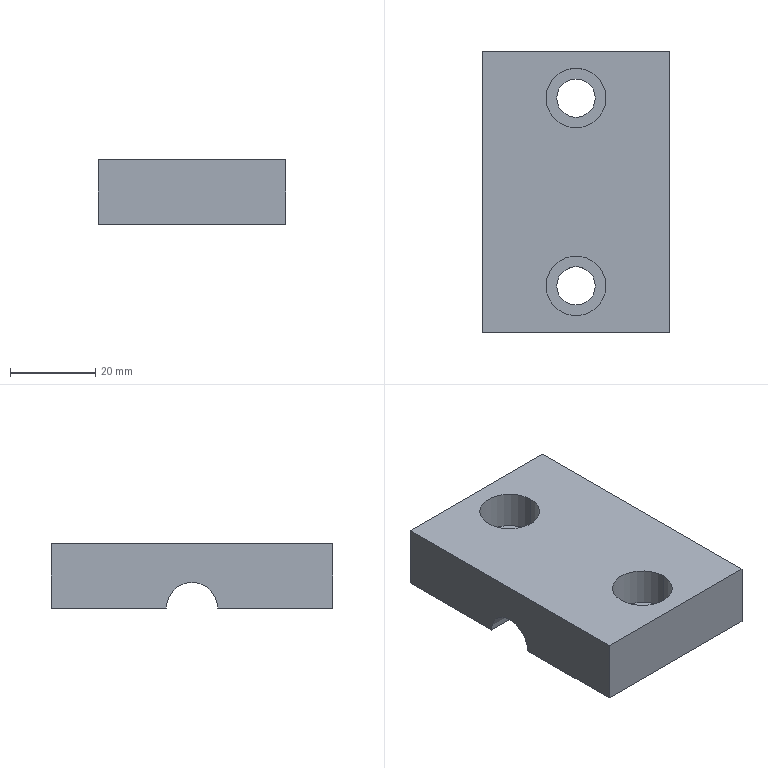Part | 1 solid | 18 faces | box 44 x 66 x 15 mm | volume 37538 mm3 | plane 9 | cylinder 9 | commonest cylinder face diameters 9 x4 14 x4 12 x1
STEP:
#1=CARTESIAN_POINT('',(0.,0.,0.));
#2=DIRECTION('',(0.,0.,1.));
#3=DIRECTION('',(1.,0.,0.));
#4=AXIS2_PLACEMENT_3D('',#1,#2,#3);
#5=CARTESIAN_POINT('',(-499.933,163.5,-310.6));
#6=VERTEX_POINT('',#5);
#7=CARTESIAN_POINT('',(-508.933,163.5,-310.6));
#8=VERTEX_POINT('',#7);
#9=CARTESIAN_POINT('',(-504.433,163.5,-310.6));
#10=DIRECTION('',(0.,0.,-1.));
#11=DIRECTION('',(-1.,0.,0.));
#12=AXIS2_PLACEMENT_3D('',#9,#10,#11);
#13=CIRCLE('',#12,4.5);
#14=CARTESIAN_POINT('',(-504.433,141.5,-310.6));
#15=DIRECTION('',(0.,0.,1.));
#16=DIRECTION('',(-1.,0.,0.));
#17=AXIS2_PLACEMENT_3D('',#14,#15,#16);
#18=PLANE('',#17);
#19=CARTESIAN_POINT('',(4.5,-22.));
#20=CARTESIAN_POINT('',(4.5,-29.794));
#21=CARTESIAN_POINT('',(-2.25,-25.897));
#22=CARTESIAN_POINT('',(-9.,-22.));
#23=CARTESIAN_POINT('',(-2.25,-18.103));
#24=CARTESIAN_POINT('',(4.5,-14.206));
#25=CARTESIAN_POINT('',(4.5,-22.));
#26=(BOUNDED_CURVE()B_SPLINE_CURVE(2,(#19,#20,#21,#22,#23,#24,#25),.UNSPECIFIED.,.T.,.F.)B_SPLINE_CURVE_WITH_KNOTS((1,2,2,2,2,1),(-2.094,0.,2.094,4.189,6.283,8.378),.UNSPECIFIED.)CURVE()GEOMETRIC_REPRESENTATION_ITEM()RATIONAL_B_SPLINE_CURVE((1.,0.5,1.,0.5,1.,0.5,1.))REPRESENTATION_ITEM(''));
#27=(GEOMETRIC_REPRESENTATION_CONTEXT(2)PARAMETRIC_REPRESENTATION_CONTEXT()REPRESENTATION_CONTEXT('',''));
#28=DEFINITIONAL_REPRESENTATION('',(#26),#27);
#29=PCURVE('',#18,#28);
#30=CARTESIAN_POINT('',(-504.433,163.5,-422.6));
#31=DIRECTION('',(0.,0.,1.));
#32=DIRECTION('',(0.,1.,0.));
#33=AXIS2_PLACEMENT_3D('',#30,#31,#32);
#34=CYLINDRICAL_SURFACE('',#33,4.5);
#35=CARTESIAN_POINT('',(7.854,112.));
#36=DIRECTION('',(-1.,0.));
#37=VECTOR('',#36,1.);
#38=LINE('',#35,#37);
#39=(GEOMETRIC_REPRESENTATION_CONTEXT(2)PARAMETRIC_REPRESENTATION_CONTEXT()REPRESENTATION_CONTEXT('',''));
#40=DEFINITIONAL_REPRESENTATION('',(#38),#39);
#41=PCURVE('',#34,#40);
#42=SURFACE_CURVE('',#13,(#29,#41),.PCURVE_S1.);
#43=EDGE_CURVE('',#6,#8,#42,.T.);
#44=ORIENTED_EDGE('',*,*,#43,.F.);
#45=CARTESIAN_POINT('',(-504.433,163.5,-310.6));
#46=DIRECTION('',(0.,0.,-1.));
#47=DIRECTION('',(-1.,0.,0.));
#48=AXIS2_PLACEMENT_3D('',#45,#46,#47);
#49=CIRCLE('',#48,4.5);
#50=CARTESIAN_POINT('',(4.5,-22.));
#51=CARTESIAN_POINT('',(4.5,-29.794));
#52=CARTESIAN_POINT('',(-2.25,-25.897));
#53=CARTESIAN_POINT('',(-9.,-22.));
#54=CARTESIAN_POINT('',(-2.25,-18.103));
#55=CARTESIAN_POINT('',(4.5,-14.206));
#56=CARTESIAN_POINT('',(4.5,-22.));
#57=(BOUNDED_CURVE()B_SPLINE_CURVE(2,(#50,#51,#52,#53,#54,#55,#56),.UNSPECIFIED.,.T.,.F.)B_SPLINE_CURVE_WITH_KNOTS((1,2,2,2,2,1),(-2.094,0.,2.094,4.189,6.283,8.378),.UNSPECIFIED.)CURVE()GEOMETRIC_REPRESENTATION_ITEM()RATIONAL_B_SPLINE_CURVE((1.,0.5,1.,0.5,1.,0.5,1.))REPRESENTATION_ITEM(''));
#58=(GEOMETRIC_REPRESENTATION_CONTEXT(2)PARAMETRIC_REPRESENTATION_CONTEXT()REPRESENTATION_CONTEXT('',''));
#59=DEFINITIONAL_REPRESENTATION('',(#57),#58);
#60=PCURVE('',#18,#59);
#61=CARTESIAN_POINT('',(-504.433,163.5,-422.6));
#62=DIRECTION('',(0.,0.,1.));
#63=DIRECTION('',(0.,-1.,0.));
#64=AXIS2_PLACEMENT_3D('',#61,#62,#63);
#65=CYLINDRICAL_SURFACE('',#64,4.5);
#66=CARTESIAN_POINT('',(4.712,112.));
#67=DIRECTION('',(-1.,0.));
#68=VECTOR('',#67,1.);
#69=LINE('',#66,#68);
#70=(GEOMETRIC_REPRESENTATION_CONTEXT(2)PARAMETRIC_REPRESENTATION_CONTEXT()REPRESENTATION_CONTEXT('',''));
#71=DEFINITIONAL_REPRESENTATION('',(#69),#70);
#72=PCURVE('',#65,#71);
#73=SURFACE_CURVE('',#49,(#60,#72),.PCURVE_S1.);
#74=EDGE_CURVE('',#8,#6,#73,.T.);
#75=ORIENTED_EDGE('',*,*,#74,.F.);
#76=EDGE_LOOP('',(#44,#75));
#77=FACE_BOUND('',#76,.T.);
#78=CARTESIAN_POINT('',(-482.433,147.5,-310.6));
#79=VERTEX_POINT('',#78);
#80=CARTESIAN_POINT('',(-482.433,174.5,-310.6));
#81=VERTEX_POINT('',#80);
#82=CARTESIAN_POINT('',(-482.433,141.5,-310.6));
#83=DIRECTION('',(0.,1.,0.));
#84=VECTOR('',#83,1.);
#85=LINE('',#82,#84);
#86=CARTESIAN_POINT('',(-22.,0.));
#87=DIRECTION('',(0.,-1.));
#88=VECTOR('',#87,1.);
#89=LINE('',#86,#88);
#90=(GEOMETRIC_REPRESENTATION_CONTEXT(2)PARAMETRIC_REPRESENTATION_CONTEXT()REPRESENTATION_CONTEXT('',''));
#91=DEFINITIONAL_REPRESENTATION('',(#89),#90);
#92=PCURVE('',#18,#91);
#93=CARTESIAN_POINT('',(-482.433,141.5,-319.1));
#94=DIRECTION('',(1.,0.,0.));
#95=DIRECTION('',(0.,0.,1.));
#96=AXIS2_PLACEMENT_3D('',#93,#94,#95);
#97=PLANE('',#96);
#98=CARTESIAN_POINT('',(8.5,0.));
#99=DIRECTION('',(0.,-1.));
#100=VECTOR('',#99,1.);
#101=LINE('',#98,#100);
#102=(GEOMETRIC_REPRESENTATION_CONTEXT(2)PARAMETRIC_REPRESENTATION_CONTEXT()REPRESENTATION_CONTEXT('',''));
#103=DEFINITIONAL_REPRESENTATION('',(#101),#102);
#104=PCURVE('',#97,#103);
#105=SURFACE_CURVE('',#85,(#92,#104),.PCURVE_S1.);
#106=EDGE_CURVE('',#79,#81,#105,.T.);
#107=ORIENTED_EDGE('',*,*,#106,.F.);
#108=CARTESIAN_POINT('',(-526.433,147.5,-310.6));
#109=VERTEX_POINT('',#108);
#110=CARTESIAN_POINT('',(-517.416,147.5,-310.6));
#111=DIRECTION('',(-1.,0.,0.));
#112=VECTOR('',#111,1.);
#113=LINE('',#110,#112);
#114=CARTESIAN_POINT('',(12.983,-6.));
#115=DIRECTION('',(1.,0.));
#116=VECTOR('',#115,1.);
#117=LINE('',#114,#116);
#118=(GEOMETRIC_REPRESENTATION_CONTEXT(2)PARAMETRIC_REPRESENTATION_CONTEXT()REPRESENTATION_CONTEXT('',''));
#119=DEFINITIONAL_REPRESENTATION('',(#117),#118);
#120=PCURVE('',#18,#119);
#121=CARTESIAN_POINT('',(-517.416,141.5,-310.6));
#122=DIRECTION('',(-1.,0.,0.));
#123=DIRECTION('',(0.,0.,-1.));
#124=AXIS2_PLACEMENT_3D('',#121,#122,#123);
#125=CYLINDRICAL_SURFACE('',#124,6.);
#126=CARTESIAN_POINT('',(4.712,0.));
#127=DIRECTION('',(0.,1.));
#128=VECTOR('',#127,1.);
#129=LINE('',#126,#128);
#130=(GEOMETRIC_REPRESENTATION_CONTEXT(2)PARAMETRIC_REPRESENTATION_CONTEXT()REPRESENTATION_CONTEXT('',''));
#131=DEFINITIONAL_REPRESENTATION('',(#129),#130);
#132=PCURVE('',#125,#131);
#133=SURFACE_CURVE('',#113,(#120,#132),.PCURVE_S1.);
#134=EDGE_CURVE('',#79,#109,#133,.T.);
#135=ORIENTED_EDGE('',*,*,#134,.T.);
#136=CARTESIAN_POINT('',(-526.433,174.5,-310.6));
#137=VERTEX_POINT('',#136);
#138=CARTESIAN_POINT('',(-526.433,141.5,-310.6));
#139=DIRECTION('',(0.,-1.,0.));
#140=VECTOR('',#139,1.);
#141=LINE('',#138,#140);
#142=CARTESIAN_POINT('',(22.,0.));
#143=DIRECTION('',(0.,1.));
#144=VECTOR('',#143,1.);
#145=LINE('',#142,#144);
#146=(GEOMETRIC_REPRESENTATION_CONTEXT(2)PARAMETRIC_REPRESENTATION_CONTEXT()REPRESENTATION_CONTEXT('',''));
#147=DEFINITIONAL_REPRESENTATION('',(#145),#146);
#148=PCURVE('',#18,#147);
#149=CARTESIAN_POINT('',(-526.433,141.5,-319.1));
#150=DIRECTION('',(-1.,0.,0.));
#151=DIRECTION('',(0.,0.,-1.));
#152=AXIS2_PLACEMENT_3D('',#149,#150,#151);
#153=PLANE('',#152);
#154=CARTESIAN_POINT('',(-8.5,0.));
#155=DIRECTION('',(0.,1.));
#156=VECTOR('',#155,1.);
#157=LINE('',#154,#156);
#158=(GEOMETRIC_REPRESENTATION_CONTEXT(2)PARAMETRIC_REPRESENTATION_CONTEXT()REPRESENTATION_CONTEXT('',''));
#159=DEFINITIONAL_REPRESENTATION('',(#157),#158);
#160=PCURVE('',#153,#159);
#161=SURFACE_CURVE('',#141,(#148,#160),.PCURVE_S1.);
#162=EDGE_CURVE('',#137,#109,#161,.T.);
#163=ORIENTED_EDGE('',*,*,#162,.F.);
#164=CARTESIAN_POINT('',(-504.433,174.5,-310.6));
#165=DIRECTION('',(1.,0.,0.));
#166=VECTOR('',#165,1.);
#167=LINE('',#164,#166);
#168=CARTESIAN_POINT('',(0.,-33.));
#169=DIRECTION('',(-1.,0.));
#170=VECTOR('',#169,1.);
#171=LINE('',#168,#170);
#172=(GEOMETRIC_REPRESENTATION_CONTEXT(2)PARAMETRIC_REPRESENTATION_CONTEXT()REPRESENTATION_CONTEXT('',''));
#173=DEFINITIONAL_REPRESENTATION('',(#171),#172);
#174=PCURVE('',#18,#173);
#175=CARTESIAN_POINT('',(-504.433,174.5,-319.1));
#176=DIRECTION('',(0.,1.,0.));
#177=DIRECTION('',(0.,0.,-1.));
#178=AXIS2_PLACEMENT_3D('',#175,#176,#177);
#179=PLANE('',#178);
#180=CARTESIAN_POINT('',(-8.5,0.));
#181=DIRECTION('',(0.,-1.));
#182=VECTOR('',#181,1.);
#183=LINE('',#180,#182);
#184=(GEOMETRIC_REPRESENTATION_CONTEXT(2)PARAMETRIC_REPRESENTATION_CONTEXT()REPRESENTATION_CONTEXT('',''));
#185=DEFINITIONAL_REPRESENTATION('',(#183),#184);
#186=PCURVE('',#179,#185);
#187=SURFACE_CURVE('',#167,(#174,#186),.PCURVE_S1.);
#188=EDGE_CURVE('',#137,#81,#187,.T.);
#189=ORIENTED_EDGE('',*,*,#188,.T.);
#190=EDGE_LOOP('',(#107,#135,#163,#189));
#191=FACE_BOUND('',#190,.T.);
#192=ADVANCED_FACE('',(#77,#191),#18,.F.);
#193=ORIENTED_EDGE('',*,*,#188,.F.);
#194=CARTESIAN_POINT('',(-526.433,174.5,-295.6));
#195=VERTEX_POINT('',#194);
#196=CARTESIAN_POINT('',(-526.433,174.5,-319.1));
#197=DIRECTION('',(0.,0.,1.));
#198=VECTOR('',#197,1.);
#199=LINE('',#196,#198);
#200=CARTESIAN_POINT('',(0.,22.));
#201=DIRECTION('',(-1.,0.));
#202=VECTOR('',#201,1.);
#203=LINE('',#200,#202);
#204=(GEOMETRIC_REPRESENTATION_CONTEXT(2)PARAMETRIC_REPRESENTATION_CONTEXT()REPRESENTATION_CONTEXT('',''));
#205=DEFINITIONAL_REPRESENTATION('',(#203),#204);
#206=PCURVE('',#179,#205);
#207=CARTESIAN_POINT('',(0.,-33.));
#208=DIRECTION('',(-1.,0.));
#209=VECTOR('',#208,1.);
#210=LINE('',#207,#209);
#211=(GEOMETRIC_REPRESENTATION_CONTEXT(2)PARAMETRIC_REPRESENTATION_CONTEXT()REPRESENTATION_CONTEXT('',''));
#212=DEFINITIONAL_REPRESENTATION('',(#210),#211);
#213=PCURVE('',#153,#212);
#214=SURFACE_CURVE('',#199,(#206,#213),.PCURVE_S1.);
#215=EDGE_CURVE('',#137,#195,#214,.T.);
#216=ORIENTED_EDGE('',*,*,#215,.T.);
#217=CARTESIAN_POINT('',(-482.433,174.5,-295.6));
#218=VERTEX_POINT('',#217);
#219=CARTESIAN_POINT('',(-504.433,174.5,-295.6));
#220=DIRECTION('',(1.,0.,0.));
#221=VECTOR('',#220,1.);
#222=LINE('',#219,#221);
#223=CARTESIAN_POINT('',(-23.5,0.));
#224=DIRECTION('',(0.,-1.));
#225=VECTOR('',#224,1.);
#226=LINE('',#223,#225);
#227=(GEOMETRIC_REPRESENTATION_CONTEXT(2)PARAMETRIC_REPRESENTATION_CONTEXT()REPRESENTATION_CONTEXT('',''));
#228=DEFINITIONAL_REPRESENTATION('',(#226),#227);
#229=PCURVE('',#179,#228);
#230=CARTESIAN_POINT('',(-504.433,141.5,-295.6));
#231=DIRECTION('',(0.,0.,1.));
#232=DIRECTION('',(-1.,0.,0.));
#233=AXIS2_PLACEMENT_3D('',#230,#231,#232);
#234=PLANE('',#233);
#235=CARTESIAN_POINT('',(0.,-33.));
#236=DIRECTION('',(-1.,0.));
#237=VECTOR('',#236,1.);
#238=LINE('',#235,#237);
#239=(GEOMETRIC_REPRESENTATION_CONTEXT(2)PARAMETRIC_REPRESENTATION_CONTEXT()REPRESENTATION_CONTEXT('',''));
#240=DEFINITIONAL_REPRESENTATION('',(#238),#239);
#241=PCURVE('',#234,#240);
#242=SURFACE_CURVE('',#222,(#229,#241),.PCURVE_S1.);
#243=EDGE_CURVE('',#195,#218,#242,.T.);
#244=ORIENTED_EDGE('',*,*,#243,.T.);
#245=CARTESIAN_POINT('',(-482.433,174.5,-319.1));
#246=DIRECTION('',(0.,0.,1.));
#247=VECTOR('',#246,1.);
#248=LINE('',#245,#247);
#249=CARTESIAN_POINT('',(0.,-22.));
#250=DIRECTION('',(-1.,0.));
#251=VECTOR('',#250,1.);
#252=LINE('',#249,#251);
#253=(GEOMETRIC_REPRESENTATION_CONTEXT(2)PARAMETRIC_REPRESENTATION_CONTEXT()REPRESENTATION_CONTEXT('',''));
#254=DEFINITIONAL_REPRESENTATION('',(#252),#253);
#255=PCURVE('',#179,#254);
#256=CARTESIAN_POINT('',(0.,-33.));
#257=DIRECTION('',(1.,0.));
#258=VECTOR('',#257,1.);
#259=LINE('',#256,#258);
#260=(GEOMETRIC_REPRESENTATION_CONTEXT(2)PARAMETRIC_REPRESENTATION_CONTEXT()REPRESENTATION_CONTEXT('',''));
#261=DEFINITIONAL_REPRESENTATION('',(#259),#260);
#262=PCURVE('',#97,#261);
#263=SURFACE_CURVE('',#248,(#255,#262),.PCURVE_S1.);
#264=EDGE_CURVE('',#81,#218,#263,.T.);
#265=ORIENTED_EDGE('',*,*,#264,.F.);
#266=EDGE_LOOP('',(#193,#216,#244,#265));
#267=FACE_BOUND('',#266,.T.);
#268=ADVANCED_FACE('',(#267),#179,.T.);
#269=CARTESIAN_POINT('',(-482.433,108.5,-310.6));
#270=VERTEX_POINT('',#269);
#271=CARTESIAN_POINT('',(-482.433,135.5,-310.6));
#272=VERTEX_POINT('',#271);
#273=CARTESIAN_POINT('',(-482.433,141.5,-310.6));
#274=DIRECTION('',(0.,1.,0.));
#275=VECTOR('',#274,1.);
#276=LINE('',#273,#275);
#277=CARTESIAN_POINT('',(8.5,0.));
#278=DIRECTION('',(0.,-1.));
#279=VECTOR('',#278,1.);
#280=LINE('',#277,#279);
#281=(GEOMETRIC_REPRESENTATION_CONTEXT(2)PARAMETRIC_REPRESENTATION_CONTEXT()REPRESENTATION_CONTEXT('',''));
#282=DEFINITIONAL_REPRESENTATION('',(#280),#281);
#283=PCURVE('',#97,#282);
#284=CARTESIAN_POINT('',(-504.433,141.5,-310.6));
#285=DIRECTION('',(0.,0.,1.));
#286=DIRECTION('',(-1.,0.,0.));
#287=AXIS2_PLACEMENT_3D('',#284,#285,#286);
#288=PLANE('',#287);
#289=CARTESIAN_POINT('',(-22.,0.));
#290=DIRECTION('',(0.,-1.));
#291=VECTOR('',#290,1.);
#292=LINE('',#289,#291);
#293=(GEOMETRIC_REPRESENTATION_CONTEXT(2)PARAMETRIC_REPRESENTATION_CONTEXT()REPRESENTATION_CONTEXT('',''));
#294=DEFINITIONAL_REPRESENTATION('',(#292),#293);
#295=PCURVE('',#288,#294);
#296=SURFACE_CURVE('',#276,(#283,#295),.PCURVE_S1.);
#297=EDGE_CURVE('',#270,#272,#296,.T.);
#298=ORIENTED_EDGE('',*,*,#297,.T.);
#299=CARTESIAN_POINT('',(-482.433,141.5,-310.6));
#300=DIRECTION('',(1.,0.,0.));
#301=DIRECTION('',(0.,0.,-1.));
#302=AXIS2_PLACEMENT_3D('',#299,#300,#301);
#303=CIRCLE('',#302,6.);
#304=CARTESIAN_POINT('',(8.5,0.));
#305=DIRECTION('',(-1.,0.));
#306=AXIS2_PLACEMENT_2D('',#304,#305);
#307=CIRCLE('',#306,6.);
#308=(GEOMETRIC_REPRESENTATION_CONTEXT(2)PARAMETRIC_REPRESENTATION_CONTEXT()REPRESENTATION_CONTEXT('',''));
#309=DEFINITIONAL_REPRESENTATION('',(#307),#308);
#310=PCURVE('',#97,#309);
#311=CARTESIAN_POINT('',(6.283,-34.983));
#312=DIRECTION('',(-1.,0.));
#313=VECTOR('',#312,1.);
#314=LINE('',#311,#313);
#315=(GEOMETRIC_REPRESENTATION_CONTEXT(2)PARAMETRIC_REPRESENTATION_CONTEXT()REPRESENTATION_CONTEXT('',''));
#316=DEFINITIONAL_REPRESENTATION('',(#314),#315);
#317=PCURVE('',#125,#316);
#318=SURFACE_CURVE('',#303,(#310,#317),.PCURVE_S1.);
#319=EDGE_CURVE('',#79,#272,#318,.T.);
#320=ORIENTED_EDGE('',*,*,#319,.F.);
#321=ORIENTED_EDGE('',*,*,#106,.T.);
#322=ORIENTED_EDGE('',*,*,#264,.T.);
#323=CARTESIAN_POINT('',(-482.433,108.5,-295.6));
#324=VERTEX_POINT('',#323);
#325=CARTESIAN_POINT('',(-482.433,141.5,-295.6));
#326=DIRECTION('',(0.,1.,0.));
#327=VECTOR('',#326,1.);
#328=LINE('',#325,#327);
#329=CARTESIAN_POINT('',(23.5,0.));
#330=DIRECTION('',(0.,-1.));
#331=VECTOR('',#330,1.);
#332=LINE('',#329,#331);
#333=(GEOMETRIC_REPRESENTATION_CONTEXT(2)PARAMETRIC_REPRESENTATION_CONTEXT()REPRESENTATION_CONTEXT('',''));
#334=DEFINITIONAL_REPRESENTATION('',(#332),#333);
#335=PCURVE('',#97,#334);
#336=CARTESIAN_POINT('',(-22.,0.));
#337=DIRECTION('',(0.,-1.));
#338=VECTOR('',#337,1.);
#339=LINE('',#336,#338);
#340=(GEOMETRIC_REPRESENTATION_CONTEXT(2)PARAMETRIC_REPRESENTATION_CONTEXT()REPRESENTATION_CONTEXT('',''));
#341=DEFINITIONAL_REPRESENTATION('',(#339),#340);
#342=PCURVE('',#234,#341);
#343=SURFACE_CURVE('',#328,(#335,#342),.PCURVE_S1.);
#344=EDGE_CURVE('',#324,#218,#343,.T.);
#345=ORIENTED_EDGE('',*,*,#344,.F.);
#346=CARTESIAN_POINT('',(-482.433,108.5,-319.1));
#347=DIRECTION('',(0.,0.,1.));
#348=VECTOR('',#347,1.);
#349=LINE('',#346,#348);
#350=CARTESIAN_POINT('',(0.,33.));
#351=DIRECTION('',(1.,0.));
#352=VECTOR('',#351,1.);
#353=LINE('',#350,#352);
#354=(GEOMETRIC_REPRESENTATION_CONTEXT(2)PARAMETRIC_REPRESENTATION_CONTEXT()REPRESENTATION_CONTEXT('',''));
#355=DEFINITIONAL_REPRESENTATION('',(#353),#354);
#356=PCURVE('',#97,#355);
#357=CARTESIAN_POINT('',(-504.433,108.5,-319.1));
#358=DIRECTION('',(0.,-1.,0.));
#359=DIRECTION('',(0.,0.,-1.));
#360=AXIS2_PLACEMENT_3D('',#357,#358,#359);
#361=PLANE('',#360);
#362=CARTESIAN_POINT('',(0.,22.));
#363=DIRECTION('',(-1.,0.));
#364=VECTOR('',#363,1.);
#365=LINE('',#362,#364);
#366=(GEOMETRIC_REPRESENTATION_CONTEXT(2)PARAMETRIC_REPRESENTATION_CONTEXT()REPRESENTATION_CONTEXT('',''));
#367=DEFINITIONAL_REPRESENTATION('',(#365),#366);
#368=PCURVE('',#361,#367);
#369=SURFACE_CURVE('',#349,(#356,#368),.PCURVE_S1.);
#370=EDGE_CURVE('',#270,#324,#369,.T.);
#371=ORIENTED_EDGE('',*,*,#370,.F.);
#372=EDGE_LOOP('',(#298,#320,#321,#322,#345,#371));
#373=FACE_BOUND('',#372,.T.);
#374=ADVANCED_FACE('',(#373),#97,.T.);
#375=CARTESIAN_POINT('',(-526.433,108.5,-310.6));
#376=VERTEX_POINT('',#375);
#377=CARTESIAN_POINT('',(-504.433,108.5,-310.6));
#378=DIRECTION('',(1.,0.,0.));
#379=VECTOR('',#378,1.);
#380=LINE('',#377,#379);
#381=CARTESIAN_POINT('',(-8.5,0.));
#382=DIRECTION('',(0.,1.));
#383=VECTOR('',#382,1.);
#384=LINE('',#381,#383);
#385=(GEOMETRIC_REPRESENTATION_CONTEXT(2)PARAMETRIC_REPRESENTATION_CONTEXT()REPRESENTATION_CONTEXT('',''));
#386=DEFINITIONAL_REPRESENTATION('',(#384),#385);
#387=PCURVE('',#361,#386);
#388=CARTESIAN_POINT('',(0.,33.));
#389=DIRECTION('',(-1.,0.));
#390=VECTOR('',#389,1.);
#391=LINE('',#388,#390);
#392=(GEOMETRIC_REPRESENTATION_CONTEXT(2)PARAMETRIC_REPRESENTATION_CONTEXT()REPRESENTATION_CONTEXT('',''));
#393=DEFINITIONAL_REPRESENTATION('',(#391),#392);
#394=PCURVE('',#288,#393);
#395=SURFACE_CURVE('',#380,(#387,#394),.PCURVE_S1.);
#396=EDGE_CURVE('',#376,#270,#395,.T.);
#397=ORIENTED_EDGE('',*,*,#396,.T.);
#398=ORIENTED_EDGE('',*,*,#370,.T.);
#399=CARTESIAN_POINT('',(-526.433,108.5,-295.6));
#400=VERTEX_POINT('',#399);
#401=CARTESIAN_POINT('',(-504.433,108.5,-295.6));
#402=DIRECTION('',(1.,0.,0.));
#403=VECTOR('',#402,1.);
#404=LINE('',#401,#403);
#405=CARTESIAN_POINT('',(-23.5,0.));
#406=DIRECTION('',(0.,1.));
#407=VECTOR('',#406,1.);
#408=LINE('',#405,#407);
#409=(GEOMETRIC_REPRESENTATION_CONTEXT(2)PARAMETRIC_REPRESENTATION_CONTEXT()REPRESENTATION_CONTEXT('',''));
#410=DEFINITIONAL_REPRESENTATION('',(#408),#409);
#411=PCURVE('',#361,#410);
#412=CARTESIAN_POINT('',(0.,33.));
#413=DIRECTION('',(-1.,0.));
#414=VECTOR('',#413,1.);
#415=LINE('',#412,#414);
#416=(GEOMETRIC_REPRESENTATION_CONTEXT(2)PARAMETRIC_REPRESENTATION_CONTEXT()REPRESENTATION_CONTEXT('',''));
#417=DEFINITIONAL_REPRESENTATION('',(#415),#416);
#418=PCURVE('',#234,#417);
#419=SURFACE_CURVE('',#404,(#411,#418),.PCURVE_S1.);
#420=EDGE_CURVE('',#400,#324,#419,.T.);
#421=ORIENTED_EDGE('',*,*,#420,.F.);
#422=CARTESIAN_POINT('',(-526.433,108.5,-319.1));
#423=DIRECTION('',(0.,0.,1.));
#424=VECTOR('',#423,1.);
#425=LINE('',#422,#424);
#426=CARTESIAN_POINT('',(0.,-22.));
#427=DIRECTION('',(-1.,0.));
#428=VECTOR('',#427,1.);
#429=LINE('',#426,#428);
#430=(GEOMETRIC_REPRESENTATION_CONTEXT(2)PARAMETRIC_REPRESENTATION_CONTEXT()REPRESENTATION_CONTEXT('',''));
#431=DEFINITIONAL_REPRESENTATION('',(#429),#430);
#432=PCURVE('',#361,#431);
#433=CARTESIAN_POINT('',(0.,33.));
#434=DIRECTION('',(-1.,0.));
#435=VECTOR('',#434,1.);
#436=LINE('',#433,#435);
#437=(GEOMETRIC_REPRESENTATION_CONTEXT(2)PARAMETRIC_REPRESENTATION_CONTEXT()REPRESENTATION_CONTEXT('',''));
#438=DEFINITIONAL_REPRESENTATION('',(#436),#437);
#439=PCURVE('',#153,#438);
#440=SURFACE_CURVE('',#425,(#432,#439),.PCURVE_S1.);
#441=EDGE_CURVE('',#376,#400,#440,.T.);
#442=ORIENTED_EDGE('',*,*,#441,.F.);
#443=EDGE_LOOP('',(#397,#398,#421,#442));
#444=FACE_BOUND('',#443,.T.);
#445=ADVANCED_FACE('',(#444),#361,.T.);
#446=CARTESIAN_POINT('',(-526.433,135.5,-310.6));
#447=VERTEX_POINT('',#446);
#448=CARTESIAN_POINT('',(-526.433,141.5,-310.6));
#449=DIRECTION('',(0.,-1.,0.));
#450=VECTOR('',#449,1.);
#451=LINE('',#448,#450);
#452=CARTESIAN_POINT('',(-8.5,0.));
#453=DIRECTION('',(0.,1.));
#454=VECTOR('',#453,1.);
#455=LINE('',#452,#454);
#456=(GEOMETRIC_REPRESENTATION_CONTEXT(2)PARAMETRIC_REPRESENTATION_CONTEXT()REPRESENTATION_CONTEXT('',''));
#457=DEFINITIONAL_REPRESENTATION('',(#455),#456);
#458=PCURVE('',#153,#457);
#459=CARTESIAN_POINT('',(22.,0.));
#460=DIRECTION('',(0.,1.));
#461=VECTOR('',#460,1.);
#462=LINE('',#459,#461);
#463=(GEOMETRIC_REPRESENTATION_CONTEXT(2)PARAMETRIC_REPRESENTATION_CONTEXT()REPRESENTATION_CONTEXT('',''));
#464=DEFINITIONAL_REPRESENTATION('',(#462),#463);
#465=PCURVE('',#288,#464);
#466=SURFACE_CURVE('',#451,(#458,#465),.PCURVE_S1.);
#467=EDGE_CURVE('',#447,#376,#466,.T.);
#468=ORIENTED_EDGE('',*,*,#467,.T.);
#469=ORIENTED_EDGE('',*,*,#441,.T.);
#470=CARTESIAN_POINT('',(-526.433,141.5,-295.6));
#471=DIRECTION('',(0.,-1.,0.));
#472=VECTOR('',#471,1.);
#473=LINE('',#470,#472);
#474=CARTESIAN_POINT('',(-23.5,0.));
#475=DIRECTION('',(0.,1.));
#476=VECTOR('',#475,1.);
#477=LINE('',#474,#476);
#478=(GEOMETRIC_REPRESENTATION_CONTEXT(2)PARAMETRIC_REPRESENTATION_CONTEXT()REPRESENTATION_CONTEXT('',''));
#479=DEFINITIONAL_REPRESENTATION('',(#477),#478);
#480=PCURVE('',#153,#479);
#481=CARTESIAN_POINT('',(22.,0.));
#482=DIRECTION('',(0.,1.));
#483=VECTOR('',#482,1.);
#484=LINE('',#481,#483);
#485=(GEOMETRIC_REPRESENTATION_CONTEXT(2)PARAMETRIC_REPRESENTATION_CONTEXT()REPRESENTATION_CONTEXT('',''));
#486=DEFINITIONAL_REPRESENTATION('',(#484),#485);
#487=PCURVE('',#234,#486);
#488=SURFACE_CURVE('',#473,(#480,#487),.PCURVE_S1.);
#489=EDGE_CURVE('',#195,#400,#488,.T.);
#490=ORIENTED_EDGE('',*,*,#489,.F.);
#491=ORIENTED_EDGE('',*,*,#215,.F.);
#492=ORIENTED_EDGE('',*,*,#162,.T.);
#493=CARTESIAN_POINT('',(-526.433,141.5,-310.6));
#494=DIRECTION('',(-1.,0.,0.));
#495=DIRECTION('',(0.,0.,1.));
#496=AXIS2_PLACEMENT_3D('',#493,#494,#495);
#497=CIRCLE('',#496,6.);
#498=CARTESIAN_POINT('',(-8.5,0.));
#499=DIRECTION('',(-1.,0.));
#500=AXIS2_PLACEMENT_2D('',#498,#499);
#501=CIRCLE('',#500,6.);
#502=(GEOMETRIC_REPRESENTATION_CONTEXT(2)PARAMETRIC_REPRESENTATION_CONTEXT()REPRESENTATION_CONTEXT('',''));
#503=DEFINITIONAL_REPRESENTATION('',(#501),#502);
#504=PCURVE('',#153,#503);
#505=CARTESIAN_POINT('',(-3.142,9.017));
#506=DIRECTION('',(1.,0.));
#507=VECTOR('',#506,1.);
#508=LINE('',#505,#507);
#509=(GEOMETRIC_REPRESENTATION_CONTEXT(2)PARAMETRIC_REPRESENTATION_CONTEXT()REPRESENTATION_CONTEXT('',''));
#510=DEFINITIONAL_REPRESENTATION('',(#508),#509);
#511=PCURVE('',#125,#510);
#512=SURFACE_CURVE('',#497,(#504,#511),.PCURVE_S1.);
#513=EDGE_CURVE('',#447,#109,#512,.T.);
#514=ORIENTED_EDGE('',*,*,#513,.F.);
#515=EDGE_LOOP('',(#468,#469,#490,#491,#492,#514));
#516=FACE_BOUND('',#515,.T.);
#517=ADVANCED_FACE('',(#516),#153,.T.);
#518=ORIENTED_EDGE('',*,*,#134,.T.);
#519=ORIENTED_EDGE('',*,*,#513,.F.);
#520=CARTESIAN_POINT('',(-517.416,135.5,-310.6));
#521=DIRECTION('',(1.,0.,0.));
#522=VECTOR('',#521,1.);
#523=LINE('',#520,#522);
#524=CARTESIAN_POINT('',(1.571,0.));
#525=DIRECTION('',(0.,-1.));
#526=VECTOR('',#525,1.);
#527=LINE('',#524,#526);
#528=(GEOMETRIC_REPRESENTATION_CONTEXT(2)PARAMETRIC_REPRESENTATION_CONTEXT()REPRESENTATION_CONTEXT('',''));
#529=DEFINITIONAL_REPRESENTATION('',(#527),#528);
#530=PCURVE('',#125,#529);
#531=CARTESIAN_POINT('',(12.983,6.));
#532=DIRECTION('',(-1.,0.));
#533=VECTOR('',#532,1.);
#534=LINE('',#531,#533);
#535=(GEOMETRIC_REPRESENTATION_CONTEXT(2)PARAMETRIC_REPRESENTATION_CONTEXT()REPRESENTATION_CONTEXT('',''));
#536=DEFINITIONAL_REPRESENTATION('',(#534),#535);
#537=PCURVE('',#288,#536);
#538=SURFACE_CURVE('',#523,(#530,#537),.PCURVE_S1.);
#539=EDGE_CURVE('',#447,#272,#538,.T.);
#540=ORIENTED_EDGE('',*,*,#539,.T.);
#541=ORIENTED_EDGE('',*,*,#319,.F.);
#542=EDGE_LOOP('',(#518,#519,#540,#541));
#543=FACE_BOUND('',#542,.F.);
#544=ADVANCED_FACE('',(#543),#125,.F.);
#545=CARTESIAN_POINT('',(-508.933,119.5,-310.6));
#546=VERTEX_POINT('',#545);
#547=CARTESIAN_POINT('',(-499.933,119.5,-310.6));
#548=VERTEX_POINT('',#547);
#549=CARTESIAN_POINT('',(-504.433,119.5,-310.6));
#550=DIRECTION('',(0.,0.,1.));
#551=DIRECTION('',(-1.,0.,0.));
#552=AXIS2_PLACEMENT_3D('',#549,#550,#551);
#553=CIRCLE('',#552,4.5);
#554=CARTESIAN_POINT('',(0.,22.));
#555=DIRECTION('',(1.,0.));
#556=AXIS2_PLACEMENT_2D('',#554,#555);
#557=CIRCLE('',#556,4.5);
#558=(GEOMETRIC_REPRESENTATION_CONTEXT(2)PARAMETRIC_REPRESENTATION_CONTEXT()REPRESENTATION_CONTEXT('',''));
#559=DEFINITIONAL_REPRESENTATION('',(#557),#558);
#560=PCURVE('',#288,#559);
#561=CARTESIAN_POINT('',(-504.433,119.5,-422.6));
#562=DIRECTION('',(0.,0.,1.));
#563=DIRECTION('',(0.,1.,0.));
#564=AXIS2_PLACEMENT_3D('',#561,#562,#563);
#565=CYLINDRICAL_SURFACE('',#564,4.5);
#566=CARTESIAN_POINT('',(1.571,112.));
#567=DIRECTION('',(1.,0.));
#568=VECTOR('',#567,1.);
#569=LINE('',#566,#568);
#570=(GEOMETRIC_REPRESENTATION_CONTEXT(2)PARAMETRIC_REPRESENTATION_CONTEXT()REPRESENTATION_CONTEXT('',''));
#571=DEFINITIONAL_REPRESENTATION('',(#569),#570);
#572=PCURVE('',#565,#571);
#573=SURFACE_CURVE('',#553,(#560,#572),.PCURVE_S1.);
#574=EDGE_CURVE('',#546,#548,#573,.T.);
#575=ORIENTED_EDGE('',*,*,#574,.T.);
#576=CARTESIAN_POINT('',(-504.433,119.5,-310.6));
#577=DIRECTION('',(0.,0.,1.));
#578=DIRECTION('',(-1.,0.,0.));
#579=AXIS2_PLACEMENT_3D('',#576,#577,#578);
#580=CIRCLE('',#579,4.5);
#581=CARTESIAN_POINT('',(0.,22.));
#582=DIRECTION('',(1.,0.));
#583=AXIS2_PLACEMENT_2D('',#581,#582);
#584=CIRCLE('',#583,4.5);
#585=(GEOMETRIC_REPRESENTATION_CONTEXT(2)PARAMETRIC_REPRESENTATION_CONTEXT()REPRESENTATION_CONTEXT('',''));
#586=DEFINITIONAL_REPRESENTATION('',(#584),#585);
#587=PCURVE('',#288,#586);
#588=CARTESIAN_POINT('',(-504.433,119.5,-422.6));
#589=DIRECTION('',(0.,0.,1.));
#590=DIRECTION('',(0.,-1.,0.));
#591=AXIS2_PLACEMENT_3D('',#588,#589,#590);
#592=CYLINDRICAL_SURFACE('',#591,4.5);
#593=CARTESIAN_POINT('',(-1.571,112.));
#594=DIRECTION('',(1.,0.));
#595=VECTOR('',#594,1.);
#596=LINE('',#593,#595);
#597=(GEOMETRIC_REPRESENTATION_CONTEXT(2)PARAMETRIC_REPRESENTATION_CONTEXT()REPRESENTATION_CONTEXT('',''));
#598=DEFINITIONAL_REPRESENTATION('',(#596),#597);
#599=PCURVE('',#592,#598);
#600=SURFACE_CURVE('',#580,(#587,#599),.PCURVE_S1.);
#601=EDGE_CURVE('',#548,#546,#600,.T.);
#602=ORIENTED_EDGE('',*,*,#601,.T.);
#603=EDGE_LOOP('',(#575,#602));
#604=FACE_BOUND('',#603,.T.);
#605=ORIENTED_EDGE('',*,*,#467,.F.);
#606=ORIENTED_EDGE('',*,*,#539,.T.);
#607=ORIENTED_EDGE('',*,*,#297,.F.);
#608=ORIENTED_EDGE('',*,*,#396,.F.);
#609=EDGE_LOOP('',(#605,#606,#607,#608));
#610=FACE_BOUND('',#609,.T.);
#611=ADVANCED_FACE('',(#604,#610),#288,.F.);
#612=ORIENTED_EDGE('',*,*,#601,.T.);
#613=CARTESIAN_POINT('',(-508.933,119.5,-304.6));
#614=VERTEX_POINT('',#613);
#615=CARTESIAN_POINT('',(-508.933,119.5,-310.6));
#616=DIRECTION('',(0.,0.,1.));
#617=VECTOR('',#616,1.);
#618=LINE('',#615,#617);
#619=CARTESIAN_POINT('',(4.712,112.));
#620=DIRECTION('',(0.,1.));
#621=VECTOR('',#620,1.);
#622=LINE('',#619,#621);
#623=(GEOMETRIC_REPRESENTATION_CONTEXT(2)PARAMETRIC_REPRESENTATION_CONTEXT()REPRESENTATION_CONTEXT('',''));
#624=DEFINITIONAL_REPRESENTATION('',(#622),#623);
#625=PCURVE('',#592,#624);
#626=CARTESIAN_POINT('',(1.571,112.));
#627=DIRECTION('',(0.,1.));
#628=VECTOR('',#627,1.);
#629=LINE('',#626,#628);
#630=(GEOMETRIC_REPRESENTATION_CONTEXT(2)PARAMETRIC_REPRESENTATION_CONTEXT()REPRESENTATION_CONTEXT('',''));
#631=DEFINITIONAL_REPRESENTATION('',(#629),#630);
#632=PCURVE('',#565,#631);
#633=SURFACE_CURVE('',#618,(#625,#632),.PCURVE_S1.);
#634=EDGE_CURVE('',#546,#614,#633,.T.);
#635=ORIENTED_EDGE('',*,*,#634,.T.);
#636=CARTESIAN_POINT('',(-499.933,119.5,-304.6));
#637=VERTEX_POINT('',#636);
#638=CARTESIAN_POINT('',(-504.433,119.5,-304.6));
#639=DIRECTION('',(0.,0.,1.));
#640=DIRECTION('',(-1.,0.,0.));
#641=AXIS2_PLACEMENT_3D('',#638,#639,#640);
#642=CIRCLE('',#641,4.5);
#643=CARTESIAN_POINT('',(-1.571,118.));
#644=DIRECTION('',(1.,0.));
#645=VECTOR('',#644,1.);
#646=LINE('',#643,#645);
#647=(GEOMETRIC_REPRESENTATION_CONTEXT(2)PARAMETRIC_REPRESENTATION_CONTEXT()REPRESENTATION_CONTEXT('',''));
#648=DEFINITIONAL_REPRESENTATION('',(#646),#647);
#649=PCURVE('',#592,#648);
#650=CARTESIAN_POINT('',(-504.433,148.5,-304.6));
#651=DIRECTION('',(0.,0.,1.));
#652=DIRECTION('',(-1.,0.,0.));
#653=AXIS2_PLACEMENT_3D('',#650,#651,#652);
#654=PLANE('',#653);
#655=CARTESIAN_POINT('',(0.,29.));
#656=DIRECTION('',(1.,0.));
#657=AXIS2_PLACEMENT_2D('',#655,#656);
#658=CIRCLE('',#657,4.5);
#659=(GEOMETRIC_REPRESENTATION_CONTEXT(2)PARAMETRIC_REPRESENTATION_CONTEXT()REPRESENTATION_CONTEXT('',''));
#660=DEFINITIONAL_REPRESENTATION('',(#658),#659);
#661=PCURVE('',#654,#660);
#662=SURFACE_CURVE('',#642,(#649,#661),.PCURVE_S1.);
#663=EDGE_CURVE('',#637,#614,#662,.T.);
#664=ORIENTED_EDGE('',*,*,#663,.F.);
#665=CARTESIAN_POINT('',(-499.933,119.5,-310.6));
#666=DIRECTION('',(0.,0.,1.));
#667=VECTOR('',#666,1.);
#668=LINE('',#665,#667);
#669=CARTESIAN_POINT('',(1.571,112.));
#670=DIRECTION('',(0.,1.));
#671=VECTOR('',#670,1.);
#672=LINE('',#669,#671);
#673=(GEOMETRIC_REPRESENTATION_CONTEXT(2)PARAMETRIC_REPRESENTATION_CONTEXT()REPRESENTATION_CONTEXT('',''));
#674=DEFINITIONAL_REPRESENTATION('',(#672),#673);
#675=PCURVE('',#592,#674);
#676=CARTESIAN_POINT('',(4.712,112.));
#677=DIRECTION('',(0.,1.));
#678=VECTOR('',#677,1.);
#679=LINE('',#676,#678);
#680=(GEOMETRIC_REPRESENTATION_CONTEXT(2)PARAMETRIC_REPRESENTATION_CONTEXT()REPRESENTATION_CONTEXT('',''));
#681=DEFINITIONAL_REPRESENTATION('',(#679),#680);
#682=PCURVE('',#565,#681);
#683=SURFACE_CURVE('',#668,(#675,#682),.PCURVE_S1.);
#684=EDGE_CURVE('',#548,#637,#683,.T.);
#685=ORIENTED_EDGE('',*,*,#684,.F.);
#686=EDGE_LOOP('',(#612,#635,#664,#685));
#687=FACE_BOUND('',#686,.F.);
#688=ADVANCED_FACE('',(#687),#592,.F.);
#689=CARTESIAN_POINT('',(-497.433,119.5,-304.6));
#690=VERTEX_POINT('',#689);
#691=CARTESIAN_POINT('',(-511.433,119.5,-304.6));
#692=VERTEX_POINT('',#691);
#693=CARTESIAN_POINT('',(-504.433,119.5,-304.6));
#694=DIRECTION('',(0.,0.,-1.));
#695=DIRECTION('',(-1.,0.,0.));
#696=AXIS2_PLACEMENT_3D('',#693,#694,#695);
#697=CIRCLE('',#696,7.);
#698=CARTESIAN_POINT('',(7.,29.));
#699=CARTESIAN_POINT('',(7.,16.876));
#700=CARTESIAN_POINT('',(-3.5,22.938));
#701=CARTESIAN_POINT('',(-14.,29.));
#702=CARTESIAN_POINT('',(-3.5,35.062));
#703=CARTESIAN_POINT('',(7.,41.124));
#704=CARTESIAN_POINT('',(7.,29.));
#705=(BOUNDED_CURVE()B_SPLINE_CURVE(2,(#698,#699,#700,#701,#702,#703,#704),.UNSPECIFIED.,.T.,.F.)B_SPLINE_CURVE_WITH_KNOTS((1,2,2,2,2,1),(-2.094,0.,2.094,4.189,6.283,8.378),.UNSPECIFIED.)CURVE()GEOMETRIC_REPRESENTATION_ITEM()RATIONAL_B_SPLINE_CURVE((1.,0.5,1.,0.5,1.,0.5,1.))REPRESENTATION_ITEM(''));
#706=(GEOMETRIC_REPRESENTATION_CONTEXT(2)PARAMETRIC_REPRESENTATION_CONTEXT()REPRESENTATION_CONTEXT('',''));
#707=DEFINITIONAL_REPRESENTATION('',(#705),#706);
#708=PCURVE('',#654,#707);
#709=CARTESIAN_POINT('',(-504.433,119.5,-422.6));
#710=DIRECTION('',(0.,0.,1.));
#711=DIRECTION('',(0.,1.,0.));
#712=AXIS2_PLACEMENT_3D('',#709,#710,#711);
#713=CYLINDRICAL_SURFACE('',#712,7.);
#714=CARTESIAN_POINT('',(7.854,118.));
#715=DIRECTION('',(-1.,0.));
#716=VECTOR('',#715,1.);
#717=LINE('',#714,#716);
#718=(GEOMETRIC_REPRESENTATION_CONTEXT(2)PARAMETRIC_REPRESENTATION_CONTEXT()REPRESENTATION_CONTEXT('',''));
#719=DEFINITIONAL_REPRESENTATION('',(#717),#718);
#720=PCURVE('',#713,#719);
#721=SURFACE_CURVE('',#697,(#708,#720),.PCURVE_S1.);
#722=EDGE_CURVE('',#690,#692,#721,.T.);
#723=ORIENTED_EDGE('',*,*,#722,.F.);
#724=CARTESIAN_POINT('',(-504.433,119.5,-304.6));
#725=DIRECTION('',(0.,0.,-1.));
#726=DIRECTION('',(-1.,0.,0.));
#727=AXIS2_PLACEMENT_3D('',#724,#725,#726);
#728=CIRCLE('',#727,7.);
#729=CARTESIAN_POINT('',(7.,29.));
#730=CARTESIAN_POINT('',(7.,16.876));
#731=CARTESIAN_POINT('',(-3.5,22.938));
#732=CARTESIAN_POINT('',(-14.,29.));
#733=CARTESIAN_POINT('',(-3.5,35.062));
#734=CARTESIAN_POINT('',(7.,41.124));
#735=CARTESIAN_POINT('',(7.,29.));
#736=(BOUNDED_CURVE()B_SPLINE_CURVE(2,(#729,#730,#731,#732,#733,#734,#735),.UNSPECIFIED.,.T.,.F.)B_SPLINE_CURVE_WITH_KNOTS((1,2,2,2,2,1),(-2.094,0.,2.094,4.189,6.283,8.378),.UNSPECIFIED.)CURVE()GEOMETRIC_REPRESENTATION_ITEM()RATIONAL_B_SPLINE_CURVE((1.,0.5,1.,0.5,1.,0.5,1.))REPRESENTATION_ITEM(''));
#737=(GEOMETRIC_REPRESENTATION_CONTEXT(2)PARAMETRIC_REPRESENTATION_CONTEXT()REPRESENTATION_CONTEXT('',''));
#738=DEFINITIONAL_REPRESENTATION('',(#736),#737);
#739=PCURVE('',#654,#738);
#740=CARTESIAN_POINT('',(-504.433,119.5,-422.6));
#741=DIRECTION('',(0.,0.,1.));
#742=DIRECTION('',(0.,-1.,0.));
#743=AXIS2_PLACEMENT_3D('',#740,#741,#742);
#744=CYLINDRICAL_SURFACE('',#743,7.);
#745=CARTESIAN_POINT('',(4.712,118.));
#746=DIRECTION('',(-1.,0.));
#747=VECTOR('',#746,1.);
#748=LINE('',#745,#747);
#749=(GEOMETRIC_REPRESENTATION_CONTEXT(2)PARAMETRIC_REPRESENTATION_CONTEXT()REPRESENTATION_CONTEXT('',''));
#750=DEFINITIONAL_REPRESENTATION('',(#748),#749);
#751=PCURVE('',#744,#750);
#752=SURFACE_CURVE('',#728,(#739,#751),.PCURVE_S1.);
#753=EDGE_CURVE('',#692,#690,#752,.T.);
#754=ORIENTED_EDGE('',*,*,#753,.F.);
#755=EDGE_LOOP('',(#723,#754));
#756=FACE_BOUND('',#755,.T.);
#757=ORIENTED_EDGE('',*,*,#663,.F.);
#758=CARTESIAN_POINT('',(-504.433,119.5,-304.6));
#759=DIRECTION('',(0.,0.,1.));
#760=DIRECTION('',(-1.,0.,0.));
#761=AXIS2_PLACEMENT_3D('',#758,#759,#760);
#762=CIRCLE('',#761,4.5);
#763=CARTESIAN_POINT('',(0.,29.));
#764=DIRECTION('',(1.,0.));
#765=AXIS2_PLACEMENT_2D('',#763,#764);
#766=CIRCLE('',#765,4.5);
#767=(GEOMETRIC_REPRESENTATION_CONTEXT(2)PARAMETRIC_REPRESENTATION_CONTEXT()REPRESENTATION_CONTEXT('',''));
#768=DEFINITIONAL_REPRESENTATION('',(#766),#767);
#769=PCURVE('',#654,#768);
#770=CARTESIAN_POINT('',(1.571,118.));
#771=DIRECTION('',(1.,0.));
#772=VECTOR('',#771,1.);
#773=LINE('',#770,#772);
#774=(GEOMETRIC_REPRESENTATION_CONTEXT(2)PARAMETRIC_REPRESENTATION_CONTEXT()REPRESENTATION_CONTEXT('',''));
#775=DEFINITIONAL_REPRESENTATION('',(#773),#774);
#776=PCURVE('',#565,#775);
#777=SURFACE_CURVE('',#762,(#769,#776),.PCURVE_S1.);
#778=EDGE_CURVE('',#614,#637,#777,.T.);
#779=ORIENTED_EDGE('',*,*,#778,.F.);
#780=EDGE_LOOP('',(#757,#779));
#781=FACE_BOUND('',#780,.T.);
#782=ADVANCED_FACE('',(#756,#781),#654,.T.);
#783=ORIENTED_EDGE('',*,*,#753,.F.);
#784=CARTESIAN_POINT('',(-511.433,119.5,-295.6));
#785=VERTEX_POINT('',#784);
#786=CARTESIAN_POINT('',(-511.433,119.5,-304.6));
#787=DIRECTION('',(0.,0.,1.));
#788=VECTOR('',#787,1.);
#789=LINE('',#786,#788);
#790=CARTESIAN_POINT('',(4.712,118.));
#791=DIRECTION('',(0.,1.));
#792=VECTOR('',#791,1.);
#793=LINE('',#790,#792);
#794=(GEOMETRIC_REPRESENTATION_CONTEXT(2)PARAMETRIC_REPRESENTATION_CONTEXT()REPRESENTATION_CONTEXT('',''));
#795=DEFINITIONAL_REPRESENTATION('',(#793),#794);
#796=PCURVE('',#744,#795);
#797=CARTESIAN_POINT('',(1.571,118.));
#798=DIRECTION('',(0.,1.));
#799=VECTOR('',#798,1.);
#800=LINE('',#797,#799);
#801=(GEOMETRIC_REPRESENTATION_CONTEXT(2)PARAMETRIC_REPRESENTATION_CONTEXT()REPRESENTATION_CONTEXT('',''));
#802=DEFINITIONAL_REPRESENTATION('',(#800),#801);
#803=PCURVE('',#713,#802);
#804=SURFACE_CURVE('',#789,(#796,#803),.PCURVE_S1.);
#805=EDGE_CURVE('',#692,#785,#804,.T.);
#806=ORIENTED_EDGE('',*,*,#805,.T.);
#807=CARTESIAN_POINT('',(-497.433,119.5,-295.6));
#808=VERTEX_POINT('',#807);
#809=CARTESIAN_POINT('',(-504.433,119.5,-295.6));
#810=DIRECTION('',(0.,0.,-1.));
#811=DIRECTION('',(-1.,0.,0.));
#812=AXIS2_PLACEMENT_3D('',#809,#810,#811);
#813=CIRCLE('',#812,7.);
#814=CARTESIAN_POINT('',(4.712,127.));
#815=DIRECTION('',(-1.,0.));
#816=VECTOR('',#815,1.);
#817=LINE('',#814,#816);
#818=(GEOMETRIC_REPRESENTATION_CONTEXT(2)PARAMETRIC_REPRESENTATION_CONTEXT()REPRESENTATION_CONTEXT('',''));
#819=DEFINITIONAL_REPRESENTATION('',(#817),#818);
#820=PCURVE('',#744,#819);
#821=CARTESIAN_POINT('',(7.,22.));
#822=CARTESIAN_POINT('',(7.,9.876));
#823=CARTESIAN_POINT('',(-3.5,15.938));
#824=CARTESIAN_POINT('',(-14.,22.));
#825=CARTESIAN_POINT('',(-3.5,28.062));
#826=CARTESIAN_POINT('',(7.,34.124));
#827=CARTESIAN_POINT('',(7.,22.));
#828=(BOUNDED_CURVE()B_SPLINE_CURVE(2,(#821,#822,#823,#824,#825,#826,#827),.UNSPECIFIED.,.T.,.F.)B_SPLINE_CURVE_WITH_KNOTS((1,2,2,2,2,1),(-2.094,0.,2.094,4.189,6.283,8.378),.UNSPECIFIED.)CURVE()GEOMETRIC_REPRESENTATION_ITEM()RATIONAL_B_SPLINE_CURVE((1.,0.5,1.,0.5,1.,0.5,1.))REPRESENTATION_ITEM(''));
#829=(GEOMETRIC_REPRESENTATION_CONTEXT(2)PARAMETRIC_REPRESENTATION_CONTEXT()REPRESENTATION_CONTEXT('',''));
#830=DEFINITIONAL_REPRESENTATION('',(#828),#829);
#831=PCURVE('',#234,#830);
#832=SURFACE_CURVE('',#813,(#820,#831),.PCURVE_S1.);
#833=EDGE_CURVE('',#785,#808,#832,.T.);
#834=ORIENTED_EDGE('',*,*,#833,.T.);
#835=CARTESIAN_POINT('',(-497.433,119.5,-304.6));
#836=DIRECTION('',(0.,0.,1.));
#837=VECTOR('',#836,1.);
#838=LINE('',#835,#837);
#839=CARTESIAN_POINT('',(1.571,118.));
#840=DIRECTION('',(0.,1.));
#841=VECTOR('',#840,1.);
#842=LINE('',#839,#841);
#843=(GEOMETRIC_REPRESENTATION_CONTEXT(2)PARAMETRIC_REPRESENTATION_CONTEXT()REPRESENTATION_CONTEXT('',''));
#844=DEFINITIONAL_REPRESENTATION('',(#842),#843);
#845=PCURVE('',#744,#844);
#846=CARTESIAN_POINT('',(4.712,118.));
#847=DIRECTION('',(0.,1.));
#848=VECTOR('',#847,1.);
#849=LINE('',#846,#848);
#850=(GEOMETRIC_REPRESENTATION_CONTEXT(2)PARAMETRIC_REPRESENTATION_CONTEXT()REPRESENTATION_CONTEXT('',''));
#851=DEFINITIONAL_REPRESENTATION('',(#849),#850);
#852=PCURVE('',#713,#851);
#853=SURFACE_CURVE('',#838,(#845,#852),.PCURVE_S1.);
#854=EDGE_CURVE('',#690,#808,#853,.T.);
#855=ORIENTED_EDGE('',*,*,#854,.F.);
#856=EDGE_LOOP('',(#783,#806,#834,#855));
#857=FACE_BOUND('',#856,.F.);
#858=ADVANCED_FACE('',(#857),#744,.F.);
#859=CARTESIAN_POINT('',(-497.433,163.5,-295.6));
#860=VERTEX_POINT('',#859);
#861=CARTESIAN_POINT('',(-511.433,163.5,-295.6));
#862=VERTEX_POINT('',#861);
#863=CARTESIAN_POINT('',(-504.433,163.5,-295.6));
#864=DIRECTION('',(0.,0.,1.));
#865=DIRECTION('',(-1.,0.,0.));
#866=AXIS2_PLACEMENT_3D('',#863,#864,#865);
#867=CIRCLE('',#866,7.);
#868=CARTESIAN_POINT('',(0.,-22.));
#869=DIRECTION('',(1.,0.));
#870=AXIS2_PLACEMENT_2D('',#868,#869);
#871=CIRCLE('',#870,7.);
#872=(GEOMETRIC_REPRESENTATION_CONTEXT(2)PARAMETRIC_REPRESENTATION_CONTEXT()REPRESENTATION_CONTEXT('',''));
#873=DEFINITIONAL_REPRESENTATION('',(#871),#872);
#874=PCURVE('',#234,#873);
#875=CARTESIAN_POINT('',(-504.433,163.5,-422.6));
#876=DIRECTION('',(0.,0.,1.));
#877=DIRECTION('',(0.,-1.,0.));
#878=AXIS2_PLACEMENT_3D('',#875,#876,#877);
#879=CYLINDRICAL_SURFACE('',#878,7.);
#880=CARTESIAN_POINT('',(-1.571,127.));
#881=DIRECTION('',(1.,0.));
#882=VECTOR('',#881,1.);
#883=LINE('',#880,#882);
#884=(GEOMETRIC_REPRESENTATION_CONTEXT(2)PARAMETRIC_REPRESENTATION_CONTEXT()REPRESENTATION_CONTEXT('',''));
#885=DEFINITIONAL_REPRESENTATION('',(#883),#884);
#886=PCURVE('',#879,#885);
#887=SURFACE_CURVE('',#867,(#874,#886),.PCURVE_S1.);
#888=EDGE_CURVE('',#860,#862,#887,.T.);
#889=ORIENTED_EDGE('',*,*,#888,.F.);
#890=CARTESIAN_POINT('',(-504.433,163.5,-295.6));
#891=DIRECTION('',(0.,0.,1.));
#892=DIRECTION('',(-1.,0.,0.));
#893=AXIS2_PLACEMENT_3D('',#890,#891,#892);
#894=CIRCLE('',#893,7.);
#895=CARTESIAN_POINT('',(0.,-22.));
#896=DIRECTION('',(1.,0.));
#897=AXIS2_PLACEMENT_2D('',#895,#896);
#898=CIRCLE('',#897,7.);
#899=(GEOMETRIC_REPRESENTATION_CONTEXT(2)PARAMETRIC_REPRESENTATION_CONTEXT()REPRESENTATION_CONTEXT('',''));
#900=DEFINITIONAL_REPRESENTATION('',(#898),#899);
#901=PCURVE('',#234,#900);
#902=CARTESIAN_POINT('',(-504.433,163.5,-422.6));
#903=DIRECTION('',(0.,0.,1.));
#904=DIRECTION('',(0.,1.,0.));
#905=AXIS2_PLACEMENT_3D('',#902,#903,#904);
#906=CYLINDRICAL_SURFACE('',#905,7.);
#907=CARTESIAN_POINT('',(1.571,127.));
#908=DIRECTION('',(1.,0.));
#909=VECTOR('',#908,1.);
#910=LINE('',#907,#909);
#911=(GEOMETRIC_REPRESENTATION_CONTEXT(2)PARAMETRIC_REPRESENTATION_CONTEXT()REPRESENTATION_CONTEXT('',''));
#912=DEFINITIONAL_REPRESENTATION('',(#910),#911);
#913=PCURVE('',#906,#912);
#914=SURFACE_CURVE('',#894,(#901,#913),.PCURVE_S1.);
#915=EDGE_CURVE('',#862,#860,#914,.T.);
#916=ORIENTED_EDGE('',*,*,#915,.F.);
#917=EDGE_LOOP('',(#889,#916));
#918=FACE_BOUND('',#917,.T.);
#919=ORIENTED_EDGE('',*,*,#833,.T.);
#920=CARTESIAN_POINT('',(-504.433,119.5,-295.6));
#921=DIRECTION('',(0.,0.,-1.));
#922=DIRECTION('',(-1.,0.,0.));
#923=AXIS2_PLACEMENT_3D('',#920,#921,#922);
#924=CIRCLE('',#923,7.);
#925=CARTESIAN_POINT('',(7.,22.));
#926=CARTESIAN_POINT('',(7.,9.876));
#927=CARTESIAN_POINT('',(-3.5,15.938));
#928=CARTESIAN_POINT('',(-14.,22.));
#929=CARTESIAN_POINT('',(-3.5,28.062));
#930=CARTESIAN_POINT('',(7.,34.124));
#931=CARTESIAN_POINT('',(7.,22.));
#932=(BOUNDED_CURVE()B_SPLINE_CURVE(2,(#925,#926,#927,#928,#929,#930,#931),.UNSPECIFIED.,.T.,.F.)B_SPLINE_CURVE_WITH_KNOTS((1,2,2,2,2,1),(-2.094,0.,2.094,4.189,6.283,8.378),.UNSPECIFIED.)CURVE()GEOMETRIC_REPRESENTATION_ITEM()RATIONAL_B_SPLINE_CURVE((1.,0.5,1.,0.5,1.,0.5,1.))REPRESENTATION_ITEM(''));
#933=(GEOMETRIC_REPRESENTATION_CONTEXT(2)PARAMETRIC_REPRESENTATION_CONTEXT()REPRESENTATION_CONTEXT('',''));
#934=DEFINITIONAL_REPRESENTATION('',(#932),#933);
#935=PCURVE('',#234,#934);
#936=CARTESIAN_POINT('',(7.854,127.));
#937=DIRECTION('',(-1.,0.));
#938=VECTOR('',#937,1.);
#939=LINE('',#936,#938);
#940=(GEOMETRIC_REPRESENTATION_CONTEXT(2)PARAMETRIC_REPRESENTATION_CONTEXT()REPRESENTATION_CONTEXT('',''));
#941=DEFINITIONAL_REPRESENTATION('',(#939),#940);
#942=PCURVE('',#713,#941);
#943=SURFACE_CURVE('',#924,(#935,#942),.PCURVE_S1.);
#944=EDGE_CURVE('',#808,#785,#943,.T.);
#945=ORIENTED_EDGE('',*,*,#944,.T.);
#946=EDGE_LOOP('',(#919,#945));
#947=FACE_BOUND('',#946,.T.);
#948=ORIENTED_EDGE('',*,*,#344,.T.);
#949=ORIENTED_EDGE('',*,*,#243,.F.);
#950=ORIENTED_EDGE('',*,*,#489,.T.);
#951=ORIENTED_EDGE('',*,*,#420,.T.);
#952=EDGE_LOOP('',(#948,#949,#950,#951));
#953=FACE_BOUND('',#952,.T.);
#954=ADVANCED_FACE('',(#918,#947,#953),#234,.T.);
#955=CARTESIAN_POINT('',(-497.433,163.5,-304.6));
#956=VERTEX_POINT('',#955);
#957=CARTESIAN_POINT('',(-511.433,163.5,-304.6));
#958=VERTEX_POINT('',#957);
#959=CARTESIAN_POINT('',(-504.433,163.5,-304.6));
#960=DIRECTION('',(0.,0.,1.));
#961=DIRECTION('',(-1.,0.,0.));
#962=AXIS2_PLACEMENT_3D('',#959,#960,#961);
#963=CIRCLE('',#962,7.);
#964=CARTESIAN_POINT('',(-1.571,118.));
#965=DIRECTION('',(1.,0.));
#966=VECTOR('',#965,1.);
#967=LINE('',#964,#966);
#968=(GEOMETRIC_REPRESENTATION_CONTEXT(2)PARAMETRIC_REPRESENTATION_CONTEXT()REPRESENTATION_CONTEXT('',''));
#969=DEFINITIONAL_REPRESENTATION('',(#967),#968);
#970=PCURVE('',#879,#969);
#971=CARTESIAN_POINT('',(-504.433,134.5,-304.6));
#972=DIRECTION('',(0.,0.,1.));
#973=DIRECTION('',(-1.,0.,0.));
#974=AXIS2_PLACEMENT_3D('',#971,#972,#973);
#975=PLANE('',#974);
#976=CARTESIAN_POINT('',(0.,-29.));
#977=DIRECTION('',(1.,0.));
#978=AXIS2_PLACEMENT_2D('',#976,#977);
#979=CIRCLE('',#978,7.);
#980=(GEOMETRIC_REPRESENTATION_CONTEXT(2)PARAMETRIC_REPRESENTATION_CONTEXT()REPRESENTATION_CONTEXT('',''));
#981=DEFINITIONAL_REPRESENTATION('',(#979),#980);
#982=PCURVE('',#975,#981);
#983=SURFACE_CURVE('',#963,(#970,#982),.PCURVE_S1.);
#984=EDGE_CURVE('',#956,#958,#983,.T.);
#985=ORIENTED_EDGE('',*,*,#984,.T.);
#986=CARTESIAN_POINT('',(-511.433,163.5,-304.6));
#987=DIRECTION('',(0.,0.,1.));
#988=VECTOR('',#987,1.);
#989=LINE('',#986,#988);
#990=CARTESIAN_POINT('',(4.712,118.));
#991=DIRECTION('',(0.,1.));
#992=VECTOR('',#991,1.);
#993=LINE('',#990,#992);
#994=(GEOMETRIC_REPRESENTATION_CONTEXT(2)PARAMETRIC_REPRESENTATION_CONTEXT()REPRESENTATION_CONTEXT('',''));
#995=DEFINITIONAL_REPRESENTATION('',(#993),#994);
#996=PCURVE('',#879,#995);
#997=CARTESIAN_POINT('',(1.571,118.));
#998=DIRECTION('',(0.,1.));
#999=VECTOR('',#998,1.);
#1000=LINE('',#997,#999);
#1001=(GEOMETRIC_REPRESENTATION_CONTEXT(2)PARAMETRIC_REPRESENTATION_CONTEXT()REPRESENTATION_CONTEXT('',''));
#1002=DEFINITIONAL_REPRESENTATION('',(#1000),#1001);
#1003=PCURVE('',#906,#1002);
#1004=SURFACE_CURVE('',#989,(#996,#1003),.PCURVE_S1.);
#1005=EDGE_CURVE('',#958,#862,#1004,.T.);
#1006=ORIENTED_EDGE('',*,*,#1005,.T.);
#1007=ORIENTED_EDGE('',*,*,#888,.F.);
#1008=CARTESIAN_POINT('',(-497.433,163.5,-304.6));
#1009=DIRECTION('',(0.,0.,1.));
#1010=VECTOR('',#1009,1.);
#1011=LINE('',#1008,#1010);
#1012=CARTESIAN_POINT('',(1.571,118.));
#1013=DIRECTION('',(0.,1.));
#1014=VECTOR('',#1013,1.);
#1015=LINE('',#1012,#1014);
#1016=(GEOMETRIC_REPRESENTATION_CONTEXT(2)PARAMETRIC_REPRESENTATION_CONTEXT()REPRESENTATION_CONTEXT('',''));
#1017=DEFINITIONAL_REPRESENTATION('',(#1015),#1016);
#1018=PCURVE('',#879,#1017);
#1019=CARTESIAN_POINT('',(4.712,118.));
#1020=DIRECTION('',(0.,1.));
#1021=VECTOR('',#1020,1.);
#1022=LINE('',#1019,#1021);
#1023=(GEOMETRIC_REPRESENTATION_CONTEXT(2)PARAMETRIC_REPRESENTATION_CONTEXT()REPRESENTATION_CONTEXT('',''));
#1024=DEFINITIONAL_REPRESENTATION('',(#1022),#1023);
#1025=PCURVE('',#906,#1024);
#1026=SURFACE_CURVE('',#1011,(#1018,#1025),.PCURVE_S1.);
#1027=EDGE_CURVE('',#956,#860,#1026,.T.);
#1028=ORIENTED_EDGE('',*,*,#1027,.F.);
#1029=EDGE_LOOP('',(#985,#1006,#1007,#1028));
#1030=FACE_BOUND('',#1029,.F.);
#1031=ADVANCED_FACE('',(#1030),#879,.F.);
#1032=CARTESIAN_POINT('',(-504.433,163.5,-304.6));
#1033=DIRECTION('',(0.,0.,1.));
#1034=DIRECTION('',(-1.,0.,0.));
#1035=AXIS2_PLACEMENT_3D('',#1032,#1033,#1034);
#1036=CIRCLE('',#1035,7.);
#1037=CARTESIAN_POINT('',(0.,-29.));
#1038=DIRECTION('',(1.,0.));
#1039=AXIS2_PLACEMENT_2D('',#1037,#1038);
#1040=CIRCLE('',#1039,7.);
#1041=(GEOMETRIC_REPRESENTATION_CONTEXT(2)PARAMETRIC_REPRESENTATION_CONTEXT()REPRESENTATION_CONTEXT('',''));
#1042=DEFINITIONAL_REPRESENTATION('',(#1040),#1041);
#1043=PCURVE('',#975,#1042);
#1044=CARTESIAN_POINT('',(1.571,118.));
#1045=DIRECTION('',(1.,0.));
#1046=VECTOR('',#1045,1.);
#1047=LINE('',#1044,#1046);
#1048=(GEOMETRIC_REPRESENTATION_CONTEXT(2)PARAMETRIC_REPRESENTATION_CONTEXT()REPRESENTATION_CONTEXT('',''));
#1049=DEFINITIONAL_REPRESENTATION('',(#1047),#1048);
#1050=PCURVE('',#906,#1049);
#1051=SURFACE_CURVE('',#1036,(#1043,#1050),.PCURVE_S1.);
#1052=EDGE_CURVE('',#958,#956,#1051,.T.);
#1053=ORIENTED_EDGE('',*,*,#1052,.T.);
#1054=ORIENTED_EDGE('',*,*,#984,.T.);
#1055=EDGE_LOOP('',(#1053,#1054));
#1056=FACE_BOUND('',#1055,.T.);
#1057=CARTESIAN_POINT('',(-508.933,163.5,-304.6));
#1058=VERTEX_POINT('',#1057);
#1059=CARTESIAN_POINT('',(-499.933,163.5,-304.6));
#1060=VERTEX_POINT('',#1059);
#1061=CARTESIAN_POINT('',(-504.433,163.5,-304.6));
#1062=DIRECTION('',(0.,0.,-1.));
#1063=DIRECTION('',(-1.,0.,0.));
#1064=AXIS2_PLACEMENT_3D('',#1061,#1062,#1063);
#1065=CIRCLE('',#1064,4.5);
#1066=CARTESIAN_POINT('',(4.5,-29.));
#1067=CARTESIAN_POINT('',(4.5,-36.794));
#1068=CARTESIAN_POINT('',(-2.25,-32.897));
#1069=CARTESIAN_POINT('',(-9.,-29.));
#1070=CARTESIAN_POINT('',(-2.25,-25.103));
#1071=CARTESIAN_POINT('',(4.5,-21.206));
#1072=CARTESIAN_POINT('',(4.5,-29.));
#1073=(BOUNDED_CURVE()B_SPLINE_CURVE(2,(#1066,#1067,#1068,#1069,#1070,#1071,#1072),.UNSPECIFIED.,.T.,.F.)B_SPLINE_CURVE_WITH_KNOTS((1,2,2,2,2,1),(-2.094,0.,2.094,4.189,6.283,8.378),.UNSPECIFIED.)CURVE()GEOMETRIC_REPRESENTATION_ITEM()RATIONAL_B_SPLINE_CURVE((1.,0.5,1.,0.5,1.,0.5,1.))REPRESENTATION_ITEM(''));
#1074=(GEOMETRIC_REPRESENTATION_CONTEXT(2)PARAMETRIC_REPRESENTATION_CONTEXT()REPRESENTATION_CONTEXT('',''));
#1075=DEFINITIONAL_REPRESENTATION('',(#1073),#1074);
#1076=PCURVE('',#975,#1075);
#1077=CARTESIAN_POINT('',(4.712,118.));
#1078=DIRECTION('',(-1.,0.));
#1079=VECTOR('',#1078,1.);
#1080=LINE('',#1077,#1079);
#1081=(GEOMETRIC_REPRESENTATION_CONTEXT(2)PARAMETRIC_REPRESENTATION_CONTEXT()REPRESENTATION_CONTEXT('',''));
#1082=DEFINITIONAL_REPRESENTATION('',(#1080),#1081);
#1083=PCURVE('',#65,#1082);
#1084=SURFACE_CURVE('',#1065,(#1076,#1083),.PCURVE_S1.);
#1085=EDGE_CURVE('',#1058,#1060,#1084,.T.);
#1086=ORIENTED_EDGE('',*,*,#1085,.T.);
#1087=CARTESIAN_POINT('',(-504.433,163.5,-304.6));
#1088=DIRECTION('',(0.,0.,-1.));
#1089=DIRECTION('',(-1.,0.,0.));
#1090=AXIS2_PLACEMENT_3D('',#1087,#1088,#1089);
#1091=CIRCLE('',#1090,4.5);
#1092=CARTESIAN_POINT('',(4.5,-29.));
#1093=CARTESIAN_POINT('',(4.5,-36.794));
#1094=CARTESIAN_POINT('',(-2.25,-32.897));
#1095=CARTESIAN_POINT('',(-9.,-29.));
#1096=CARTESIAN_POINT('',(-2.25,-25.103));
#1097=CARTESIAN_POINT('',(4.5,-21.206));
#1098=CARTESIAN_POINT('',(4.5,-29.));
#1099=(BOUNDED_CURVE()B_SPLINE_CURVE(2,(#1092,#1093,#1094,#1095,#1096,#1097,#1098),.UNSPECIFIED.,.T.,.F.)B_SPLINE_CURVE_WITH_KNOTS((1,2,2,2,2,1),(-2.094,0.,2.094,4.189,6.283,8.378),.UNSPECIFIED.)CURVE()GEOMETRIC_REPRESENTATION_ITEM()RATIONAL_B_SPLINE_CURVE((1.,0.5,1.,0.5,1.,0.5,1.))REPRESENTATION_ITEM(''));
#1100=(GEOMETRIC_REPRESENTATION_CONTEXT(2)PARAMETRIC_REPRESENTATION_CONTEXT()REPRESENTATION_CONTEXT('',''));
#1101=DEFINITIONAL_REPRESENTATION('',(#1099),#1100);
#1102=PCURVE('',#975,#1101);
#1103=CARTESIAN_POINT('',(7.854,118.));
#1104=DIRECTION('',(-1.,0.));
#1105=VECTOR('',#1104,1.);
#1106=LINE('',#1103,#1105);
#1107=(GEOMETRIC_REPRESENTATION_CONTEXT(2)PARAMETRIC_REPRESENTATION_CONTEXT()REPRESENTATION_CONTEXT('',''));
#1108=DEFINITIONAL_REPRESENTATION('',(#1106),#1107);
#1109=PCURVE('',#34,#1108);
#1110=SURFACE_CURVE('',#1091,(#1102,#1109),.PCURVE_S1.);
#1111=EDGE_CURVE('',#1060,#1058,#1110,.T.);
#1112=ORIENTED_EDGE('',*,*,#1111,.T.);
#1113=EDGE_LOOP('',(#1086,#1112));
#1114=FACE_BOUND('',#1113,.T.);
#1115=ADVANCED_FACE('',(#1056,#1114),#975,.T.);
#1116=ORIENTED_EDGE('',*,*,#74,.F.);
#1117=CARTESIAN_POINT('',(-508.933,163.5,-310.6));
#1118=DIRECTION('',(0.,0.,1.));
#1119=VECTOR('',#1118,1.);
#1120=LINE('',#1117,#1119);
#1121=CARTESIAN_POINT('',(4.712,112.));
#1122=DIRECTION('',(0.,1.));
#1123=VECTOR('',#1122,1.);
#1124=LINE('',#1121,#1123);
#1125=(GEOMETRIC_REPRESENTATION_CONTEXT(2)PARAMETRIC_REPRESENTATION_CONTEXT()REPRESENTATION_CONTEXT('',''));
#1126=DEFINITIONAL_REPRESENTATION('',(#1124),#1125);
#1127=PCURVE('',#65,#1126);
#1128=CARTESIAN_POINT('',(1.571,112.));
#1129=DIRECTION('',(0.,1.));
#1130=VECTOR('',#1129,1.);
#1131=LINE('',#1128,#1130);
#1132=(GEOMETRIC_REPRESENTATION_CONTEXT(2)PARAMETRIC_REPRESENTATION_CONTEXT()REPRESENTATION_CONTEXT('',''));
#1133=DEFINITIONAL_REPRESENTATION('',(#1131),#1132);
#1134=PCURVE('',#34,#1133);
#1135=SURFACE_CURVE('',#1120,(#1127,#1134),.PCURVE_S1.);
#1136=EDGE_CURVE('',#8,#1058,#1135,.T.);
#1137=ORIENTED_EDGE('',*,*,#1136,.T.);
#1138=ORIENTED_EDGE('',*,*,#1085,.T.);
#1139=CARTESIAN_POINT('',(-499.933,163.5,-310.6));
#1140=DIRECTION('',(0.,0.,1.));
#1141=VECTOR('',#1140,1.);
#1142=LINE('',#1139,#1141);
#1143=CARTESIAN_POINT('',(1.571,112.));
#1144=DIRECTION('',(0.,1.));
#1145=VECTOR('',#1144,1.);
#1146=LINE('',#1143,#1145);
#1147=(GEOMETRIC_REPRESENTATION_CONTEXT(2)PARAMETRIC_REPRESENTATION_CONTEXT()REPRESENTATION_CONTEXT('',''));
#1148=DEFINITIONAL_REPRESENTATION('',(#1146),#1147);
#1149=PCURVE('',#65,#1148);
#1150=CARTESIAN_POINT('',(4.712,112.));
#1151=DIRECTION('',(0.,1.));
#1152=VECTOR('',#1151,1.);
#1153=LINE('',#1150,#1152);
#1154=(GEOMETRIC_REPRESENTATION_CONTEXT(2)PARAMETRIC_REPRESENTATION_CONTEXT()REPRESENTATION_CONTEXT('',''));
#1155=DEFINITIONAL_REPRESENTATION('',(#1153),#1154);
#1156=PCURVE('',#34,#1155);
#1157=SURFACE_CURVE('',#1142,(#1149,#1156),.PCURVE_S1.);
#1158=EDGE_CURVE('',#6,#1060,#1157,.T.);
#1159=ORIENTED_EDGE('',*,*,#1158,.F.);
#1160=EDGE_LOOP('',(#1116,#1137,#1138,#1159));
#1161=FACE_BOUND('',#1160,.F.);
#1162=ADVANCED_FACE('',(#1161),#65,.F.);
#1163=ORIENTED_EDGE('',*,*,#778,.F.);
#1164=ORIENTED_EDGE('',*,*,#634,.F.);
#1165=ORIENTED_EDGE('',*,*,#574,.T.);
#1166=ORIENTED_EDGE('',*,*,#684,.T.);
#1167=EDGE_LOOP('',(#1163,#1164,#1165,#1166));
#1168=FACE_BOUND('',#1167,.F.);
#1169=ADVANCED_FACE('',(#1168),#565,.F.);
#1170=ORIENTED_EDGE('',*,*,#944,.T.);
#1171=ORIENTED_EDGE('',*,*,#805,.F.);
#1172=ORIENTED_EDGE('',*,*,#722,.F.);
#1173=ORIENTED_EDGE('',*,*,#854,.T.);
#1174=EDGE_LOOP('',(#1170,#1171,#1172,#1173));
#1175=FACE_BOUND('',#1174,.F.);
#1176=ADVANCED_FACE('',(#1175),#713,.F.);
#1177=ORIENTED_EDGE('',*,*,#915,.F.);
#1178=ORIENTED_EDGE('',*,*,#1005,.F.);
#1179=ORIENTED_EDGE('',*,*,#1052,.T.);
#1180=ORIENTED_EDGE('',*,*,#1027,.T.);
#1181=EDGE_LOOP('',(#1177,#1178,#1179,#1180));
#1182=FACE_BOUND('',#1181,.F.);
#1183=ADVANCED_FACE('',(#1182),#906,.F.);
#1184=ORIENTED_EDGE('',*,*,#1111,.T.);
#1185=ORIENTED_EDGE('',*,*,#1136,.F.);
#1186=ORIENTED_EDGE('',*,*,#43,.F.);
#1187=ORIENTED_EDGE('',*,*,#1158,.T.);
#1188=EDGE_LOOP('',(#1184,#1185,#1186,#1187));
#1189=FACE_BOUND('',#1188,.F.);
#1190=ADVANCED_FACE('',(#1189),#34,.F.);
#1191=CLOSED_SHELL('',(#192,#268,#374,#445,#517,#544,#611,#688,#782,#858,#954,#1031,#1115,#1162,#1169,#1176,#1183,#1190));
#1192=MANIFOLD_SOLID_BREP('',#1191);
#1193=(LENGTH_UNIT()NAMED_UNIT(*)SI_UNIT(.MILLI.,.METRE.));
#1194=UNCERTAINTY_MEASURE_WITH_UNIT(LENGTH_MEASURE(0.0000001),#1193,'','');
#1195=(NAMED_UNIT(*)PLANE_ANGLE_UNIT()SI_UNIT($,.RADIAN.));
#1196=(NAMED_UNIT(*)SI_UNIT($,.STERADIAN.)SOLID_ANGLE_UNIT());
#1197=(GEOMETRIC_REPRESENTATION_CONTEXT(3)GLOBAL_UNCERTAINTY_ASSIGNED_CONTEXT((#1194))GLOBAL_UNIT_ASSIGNED_CONTEXT((#1193,#1195,#1196))REPRESENTATION_CONTEXT('',''));
#1198=ADVANCED_BREP_SHAPE_REPRESENTATION('',(#4,#1192),#1197);